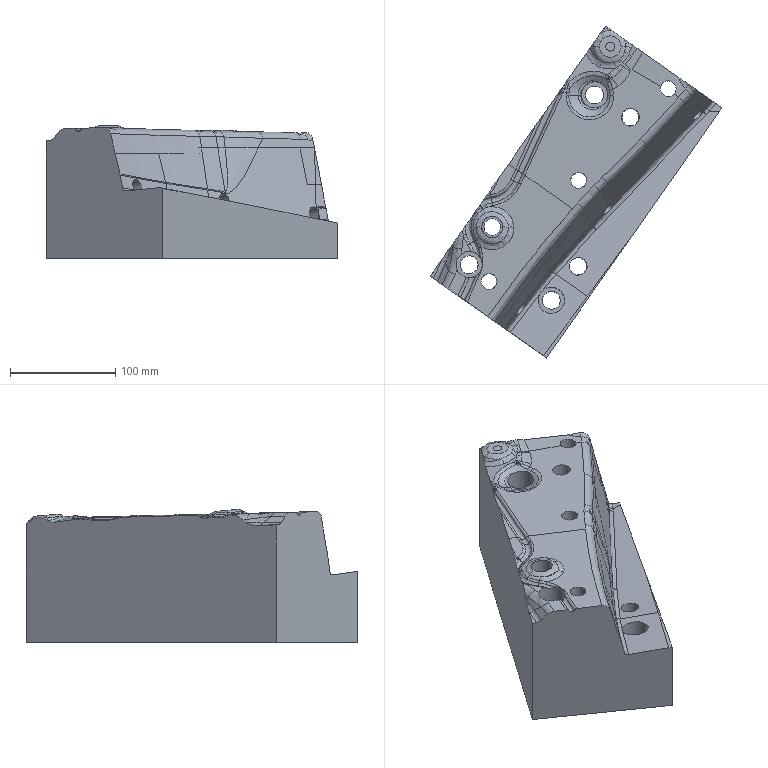Part | NX | features solid 2 | 1 solid | 207 faces | box 276.923 x 314.987 x 126.46 mm | volume 3633619 mm3 | spline 167 | cylinder 22 | plane 18 | commonest cylinder face diameters 17 x5 10 x3 13 x3 15 x3 16 x3 25 x3